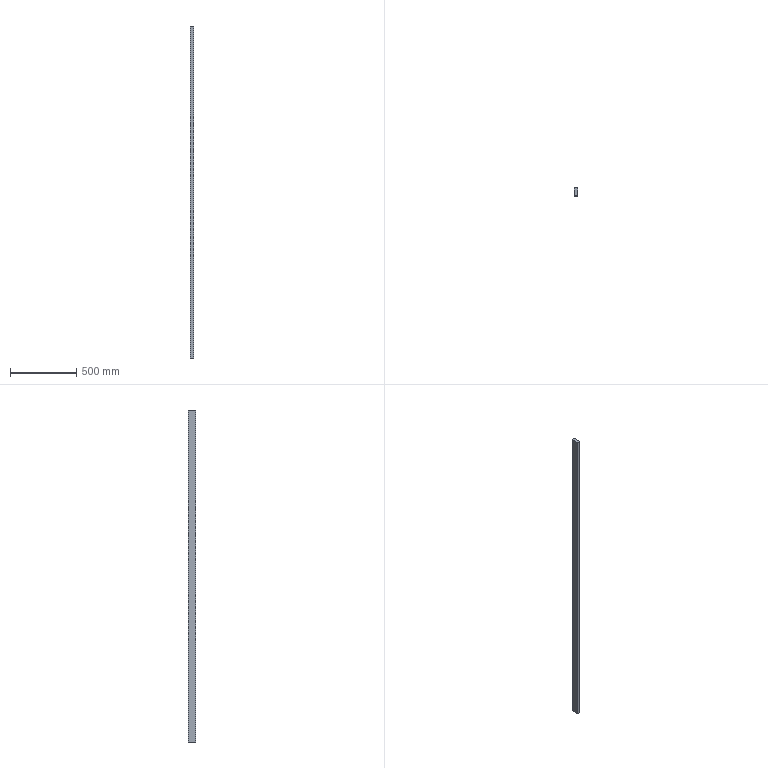Part | STEP file | Part 17 | 1 solid | 6 faces | box 25 x 60 x 2500 mm | volume 3750000 mm3 | plane 6
STEP:
#1=CARTESIAN_POINT('',(13.5,0.,-2500.));
#2=VERTEX_POINT('',#1);
#3=CARTESIAN_POINT('',(-11.5,0.,-2500.));
#4=VERTEX_POINT('',#3);
#5=CARTESIAN_POINT('',(11.5,0.,-2500.));
#6=DIRECTION('',(-1.,0.,0.));
#7=VECTOR('',#6,1000.);
#8=LINE('',#5,#7);
#9=EDGE_CURVE('',#2,#4,#8,.T.);
#10=ORIENTED_EDGE('',*,*,#9,.F.);
#11=CARTESIAN_POINT('',(13.5,-60.,-2500.));
#12=VERTEX_POINT('',#11);
#13=CARTESIAN_POINT('',(13.5,-60.,-2500.));
#14=DIRECTION('',(0.,1.,0.));
#15=VECTOR('',#14,1000.);
#16=LINE('',#13,#15);
#17=EDGE_CURVE('',#12,#2,#16,.T.);
#18=ORIENTED_EDGE('',*,*,#17,.F.);
#19=CARTESIAN_POINT('',(-11.5,-60.,-2500.));
#20=VERTEX_POINT('',#19);
#21=CARTESIAN_POINT('',(-11.5,-60.,-2500.));
#22=DIRECTION('',(1.,0.,0.));
#23=VECTOR('',#22,1000.);
#24=LINE('',#21,#23);
#25=EDGE_CURVE('',#20,#12,#24,.T.);
#26=ORIENTED_EDGE('',*,*,#25,.F.);
#27=CARTESIAN_POINT('',(-11.5,0.,-2500.));
#28=DIRECTION('',(0.,-1.,0.));
#29=VECTOR('',#28,1000.);
#30=LINE('',#27,#29);
#31=EDGE_CURVE('',#4,#20,#30,.T.);
#32=ORIENTED_EDGE('',*,*,#31,.F.);
#33=EDGE_LOOP('',(#10,#18,#26,#32));
#34=FACE_OUTER_BOUND('',#33,.T.);
#35=CARTESIAN_POINT('',(-10.995,12.455,-2500.));
#36=DIRECTION('',(0.,0.,-1.));
#37=DIRECTION('',(-1.,0.,0.));
#38=AXIS2_PLACEMENT_3D('',#35,#36,#37);
#39=PLANE('',#38);
#40=ADVANCED_FACE('',(#34),#39,.T.);
#41=CARTESIAN_POINT('',(13.5,-60.,0.));
#42=VERTEX_POINT('',#41);
#43=CARTESIAN_POINT('',(13.5,0.,0.));
#44=VERTEX_POINT('',#43);
#45=CARTESIAN_POINT('',(13.5,-60.,0.));
#46=DIRECTION('',(0.,1.,0.));
#47=VECTOR('',#46,1000.);
#48=LINE('',#45,#47);
#49=EDGE_CURVE('',#42,#44,#48,.T.);
#50=ORIENTED_EDGE('',*,*,#49,.T.);
#51=CARTESIAN_POINT('',(-11.5,0.,0.));
#52=VERTEX_POINT('',#51);
#53=CARTESIAN_POINT('',(11.5,0.,0.));
#54=DIRECTION('',(-1.,0.,0.));
#55=VECTOR('',#54,1000.);
#56=LINE('',#53,#55);
#57=EDGE_CURVE('',#44,#52,#56,.T.);
#58=ORIENTED_EDGE('',*,*,#57,.T.);
#59=CARTESIAN_POINT('',(-11.5,-60.,0.));
#60=VERTEX_POINT('',#59);
#61=CARTESIAN_POINT('',(-11.5,0.,0.));
#62=DIRECTION('',(0.,-1.,0.));
#63=VECTOR('',#62,1000.);
#64=LINE('',#61,#63);
#65=EDGE_CURVE('',#52,#60,#64,.T.);
#66=ORIENTED_EDGE('',*,*,#65,.T.);
#67=CARTESIAN_POINT('',(-11.5,-60.,0.));
#68=DIRECTION('',(1.,0.,0.));
#69=VECTOR('',#68,1000.);
#70=LINE('',#67,#69);
#71=EDGE_CURVE('',#60,#42,#70,.T.);
#72=ORIENTED_EDGE('',*,*,#71,.T.);
#73=EDGE_LOOP('',(#50,#58,#66,#72));
#74=FACE_OUTER_BOUND('',#73,.T.);
#75=CARTESIAN_POINT('',(0.,0.,0.));
#76=DIRECTION('',(0.,0.,1.));
#77=DIRECTION('',(1.,0.,0.));
#78=AXIS2_PLACEMENT_3D('',#75,#76,#77);
#79=PLANE('',#78);
#80=ADVANCED_FACE('',(#74),#79,.T.);
#81=ORIENTED_EDGE('',*,*,#57,.F.);
#82=CARTESIAN_POINT('',(13.5,0.,-2566.851));
#83=DIRECTION('',(0.,0.,-1.));
#84=VECTOR('',#83,1000.);
#85=LINE('',#82,#84);
#86=EDGE_CURVE('',#44,#2,#85,.T.);
#87=ORIENTED_EDGE('',*,*,#86,.T.);
#88=ORIENTED_EDGE('',*,*,#9,.T.);
#89=CARTESIAN_POINT('',(-11.5,0.,-2566.851));
#90=DIRECTION('',(0.,0.,1.));
#91=VECTOR('',#90,1000.);
#92=LINE('',#89,#91);
#93=EDGE_CURVE('',#4,#52,#92,.T.);
#94=ORIENTED_EDGE('',*,*,#93,.T.);
#95=EDGE_LOOP('',(#81,#87,#88,#94));
#96=FACE_OUTER_BOUND('',#95,.T.);
#97=CARTESIAN_POINT('',(11.5,0.,-2566.851));
#98=DIRECTION('',(0.,1.,0.));
#99=DIRECTION('',(-1.,0.,0.));
#100=AXIS2_PLACEMENT_3D('',#97,#98,#99);
#101=PLANE('',#100);
#102=ADVANCED_FACE('',(#96),#101,.T.);
#103=ORIENTED_EDGE('',*,*,#93,.F.);
#104=ORIENTED_EDGE('',*,*,#31,.T.);
#105=CARTESIAN_POINT('',(-11.5,-60.,-2566.851));
#106=DIRECTION('',(0.,0.,1.));
#107=VECTOR('',#106,1000.);
#108=LINE('',#105,#107);
#109=EDGE_CURVE('',#20,#60,#108,.T.);
#110=ORIENTED_EDGE('',*,*,#109,.T.);
#111=ORIENTED_EDGE('',*,*,#65,.F.);
#112=EDGE_LOOP('',(#103,#104,#110,#111));
#113=FACE_OUTER_BOUND('',#112,.T.);
#114=CARTESIAN_POINT('',(-11.5,0.,-2566.851));
#115=DIRECTION('',(-1.,0.,0.));
#116=DIRECTION('',(0.,-1.,0.));
#117=AXIS2_PLACEMENT_3D('',#114,#115,#116);
#118=PLANE('',#117);
#119=ADVANCED_FACE('',(#113),#118,.T.);
#120=ORIENTED_EDGE('',*,*,#109,.F.);
#121=ORIENTED_EDGE('',*,*,#25,.T.);
#122=CARTESIAN_POINT('',(13.5,-60.,-2566.851));
#123=DIRECTION('',(0.,0.,1.));
#124=VECTOR('',#123,1000.);
#125=LINE('',#122,#124);
#126=EDGE_CURVE('',#12,#42,#125,.T.);
#127=ORIENTED_EDGE('',*,*,#126,.T.);
#128=ORIENTED_EDGE('',*,*,#71,.F.);
#129=EDGE_LOOP('',(#120,#121,#127,#128));
#130=FACE_OUTER_BOUND('',#129,.T.);
#131=CARTESIAN_POINT('',(-11.5,-60.,-2566.851));
#132=DIRECTION('',(0.,-1.,0.));
#133=DIRECTION('',(1.,0.,0.));
#134=AXIS2_PLACEMENT_3D('',#131,#132,#133);
#135=PLANE('',#134);
#136=ADVANCED_FACE('',(#130),#135,.T.);
#137=ORIENTED_EDGE('',*,*,#86,.F.);
#138=ORIENTED_EDGE('',*,*,#49,.F.);
#139=ORIENTED_EDGE('',*,*,#126,.F.);
#140=ORIENTED_EDGE('',*,*,#17,.T.);
#141=EDGE_LOOP('',(#137,#138,#139,#140));
#142=FACE_OUTER_BOUND('',#141,.T.);
#143=CARTESIAN_POINT('',(13.5,-60.,-2566.851));
#144=DIRECTION('',(1.,0.,0.));
#145=DIRECTION('',(0.,1.,0.));
#146=AXIS2_PLACEMENT_3D('',#143,#144,#145);
#147=PLANE('',#146);
#148=ADVANCED_FACE('',(#142),#147,.T.);
#149=CLOSED_SHELL('',(#40,#80,#102,#119,#136,#148));
#150=MANIFOLD_SOLID_BREP('',#149);
#151=CARTESIAN_POINT('',(0.,0.,0.));
#152=DIRECTION('',(0.,0.,1.));
#153=DIRECTION('',(1.,0.,0.));
#154=AXIS2_PLACEMENT_3D('',#151,#152,#153);
#155=(LENGTH_UNIT()NAMED_UNIT(*)SI_UNIT(.MILLI.,.METRE.));
#156=UNCERTAINTY_MEASURE_WITH_UNIT(LENGTH_MEASURE(0.00001),#155,'','');
#157=(NAMED_UNIT(*)PLANE_ANGLE_UNIT()SI_UNIT($,.RADIAN.));
#158=(NAMED_UNIT(*)SI_UNIT($,.STERADIAN.)SOLID_ANGLE_UNIT());
#159=(GEOMETRIC_REPRESENTATION_CONTEXT(3)GLOBAL_UNCERTAINTY_ASSIGNED_CONTEXT((#156))GLOBAL_UNIT_ASSIGNED_CONTEXT((#155,#157,#158))REPRESENTATION_CONTEXT('',''));
#160=ADVANCED_BREP_SHAPE_REPRESENTATION('',(#150,#154),#159);